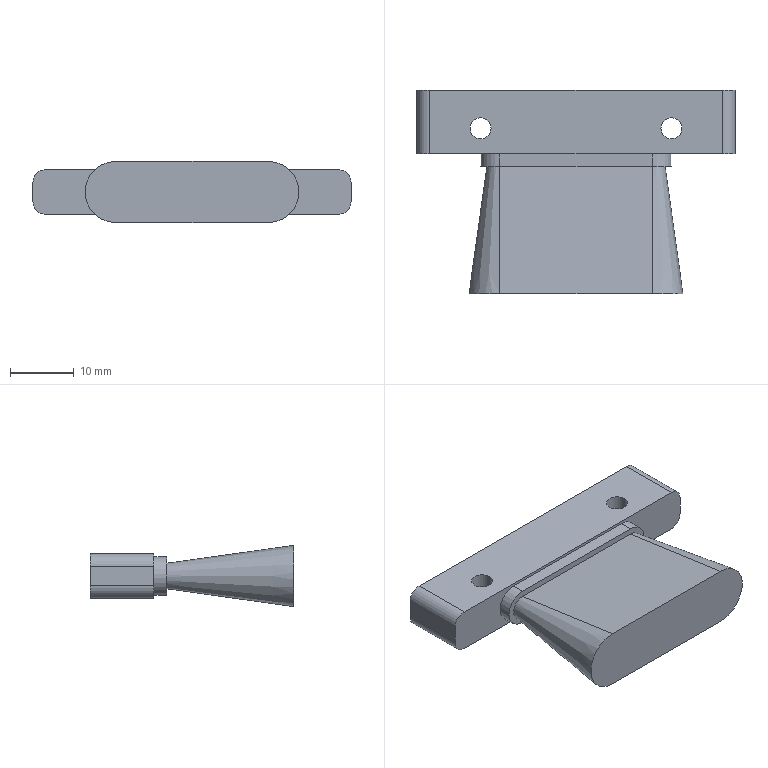Part | SolidWorks | features ICE 2, 3DProfileFeature 1, Extrusion 1, Fillet 1, HoleWzd 1 | 1 solid | 24 faces | box 50 x 32 x 9.622 mm | volume 7730 mm3 | plane 12 | cylinder 10 | cone 2 | commonest cylinder face diameters 3.3 x4 4 x4 6 x2
STEP:
#1=CARTESIAN_POINT('',(16.65,4.,3.5));
#2=VERTEX_POINT('',#1);
#3=CARTESIAN_POINT('',(13.35,4.,3.5));
#4=VERTEX_POINT('',#3);
#5=CARTESIAN_POINT('',(15.,4.,3.5));
#6=DIRECTION('',(0.,0.,-1.));
#7=DIRECTION('',(-1.,0.,0.));
#8=AXIS2_PLACEMENT_3D('',#5,#6,#7);
#9=CIRCLE('',#8,1.65);
#10=EDGE_CURVE('',#2,#4,#9,.T.);
#11=ORIENTED_EDGE('',*,*,#10,.F.);
#12=CARTESIAN_POINT('',(16.65,4.,-3.5));
#13=VERTEX_POINT('',#12);
#14=CARTESIAN_POINT('',(16.65,4.,-3.5));
#15=DIRECTION('',(0.,0.,-1.));
#16=VECTOR('',#15,1000.);
#17=LINE('',#14,#16);
#18=EDGE_CURVE('',#2,#13,#17,.T.);
#19=ORIENTED_EDGE('',*,*,#18,.T.);
#20=CARTESIAN_POINT('',(13.35,4.,-3.5));
#21=VERTEX_POINT('',#20);
#22=CARTESIAN_POINT('',(15.,4.,-3.5));
#23=DIRECTION('',(0.,0.,-1.));
#24=DIRECTION('',(-1.,0.,0.));
#25=AXIS2_PLACEMENT_3D('',#22,#23,#24);
#26=CIRCLE('',#25,1.65);
#27=EDGE_CURVE('',#13,#21,#26,.T.);
#28=ORIENTED_EDGE('',*,*,#27,.T.);
#29=CARTESIAN_POINT('',(13.35,4.,-3.5));
#30=DIRECTION('',(0.,0.,-1.));
#31=VECTOR('',#30,1000.);
#32=LINE('',#29,#31);
#33=EDGE_CURVE('',#4,#21,#32,.T.);
#34=ORIENTED_EDGE('',*,*,#33,.F.);
#35=EDGE_LOOP('',(#11,#19,#28,#34));
#36=FACE_OUTER_BOUND('',#35,.T.);
#37=CARTESIAN_POINT('',(15.,4.,-3.5));
#38=DIRECTION('',(0.,0.,-1.));
#39=DIRECTION('',(-1.,0.,0.));
#40=AXIS2_PLACEMENT_3D('',#37,#38,#39);
#41=CYLINDRICAL_SURFACE('',#40,1.65);
#42=ADVANCED_FACE('',(#36),#41,.F.);
#43=CARTESIAN_POINT('',(-13.35,4.,3.5));
#44=VERTEX_POINT('',#43);
#45=CARTESIAN_POINT('',(-16.65,4.,3.5));
#46=VERTEX_POINT('',#45);
#47=CARTESIAN_POINT('',(-15.,4.,3.5));
#48=DIRECTION('',(0.,0.,-1.));
#49=DIRECTION('',(-1.,0.,0.));
#50=AXIS2_PLACEMENT_3D('',#47,#48,#49);
#51=CIRCLE('',#50,1.65);
#52=EDGE_CURVE('',#44,#46,#51,.T.);
#53=ORIENTED_EDGE('',*,*,#52,.F.);
#54=CARTESIAN_POINT('',(-13.35,4.,-3.5));
#55=VERTEX_POINT('',#54);
#56=CARTESIAN_POINT('',(-13.35,4.,-3.5));
#57=DIRECTION('',(0.,0.,-1.));
#58=VECTOR('',#57,1000.);
#59=LINE('',#56,#58);
#60=EDGE_CURVE('',#44,#55,#59,.T.);
#61=ORIENTED_EDGE('',*,*,#60,.T.);
#62=CARTESIAN_POINT('',(-16.65,4.,-3.5));
#63=VERTEX_POINT('',#62);
#64=CARTESIAN_POINT('',(-15.,4.,-3.5));
#65=DIRECTION('',(0.,0.,-1.));
#66=DIRECTION('',(-1.,0.,0.));
#67=AXIS2_PLACEMENT_3D('',#64,#65,#66);
#68=CIRCLE('',#67,1.65);
#69=EDGE_CURVE('',#55,#63,#68,.T.);
#70=ORIENTED_EDGE('',*,*,#69,.T.);
#71=CARTESIAN_POINT('',(-16.65,4.,-3.5));
#72=DIRECTION('',(0.,0.,-1.));
#73=VECTOR('',#72,1000.);
#74=LINE('',#71,#73);
#75=EDGE_CURVE('',#46,#63,#74,.T.);
#76=ORIENTED_EDGE('',*,*,#75,.F.);
#77=EDGE_LOOP('',(#53,#61,#70,#76));
#78=FACE_OUTER_BOUND('',#77,.T.);
#79=CARTESIAN_POINT('',(-15.,4.,-3.5));
#80=DIRECTION('',(0.,0.,-1.));
#81=DIRECTION('',(-1.,0.,0.));
#82=AXIS2_PLACEMENT_3D('',#79,#80,#81);
#83=CYLINDRICAL_SURFACE('',#82,1.65);
#84=ADVANCED_FACE('',(#78),#83,.F.);
#85=CARTESIAN_POINT('',(-12.,-2.,3.));
#86=VERTEX_POINT('',#85);
#87=CARTESIAN_POINT('',(12.,-2.,3.));
#88=VERTEX_POINT('',#87);
#89=CARTESIAN_POINT('',(0.,-2.,3.));
#90=DIRECTION('',(1.,0.,0.));
#91=VECTOR('',#90,1000.);
#92=LINE('',#89,#91);
#93=EDGE_CURVE('',#86,#88,#92,.T.);
#94=ORIENTED_EDGE('',*,*,#93,.F.);
#95=CARTESIAN_POINT('',(-12.,-2.,-3.));
#96=VERTEX_POINT('',#95);
#97=CARTESIAN_POINT('',(-12.,-2.,0.));
#98=DIRECTION('',(0.,1.,0.));
#99=DIRECTION('',(0.,0.,1.));
#100=AXIS2_PLACEMENT_3D('',#97,#98,#99);
#101=CIRCLE('',#100,3.);
#102=EDGE_CURVE('',#96,#86,#101,.T.);
#103=ORIENTED_EDGE('',*,*,#102,.F.);
#104=CARTESIAN_POINT('',(12.,-2.,-3.));
#105=VERTEX_POINT('',#104);
#106=CARTESIAN_POINT('',(0.,-2.,-3.));
#107=DIRECTION('',(1.,0.,0.));
#108=VECTOR('',#107,1000.);
#109=LINE('',#106,#108);
#110=EDGE_CURVE('',#96,#105,#109,.T.);
#111=ORIENTED_EDGE('',*,*,#110,.T.);
#112=CARTESIAN_POINT('',(12.,-2.,0.));
#113=DIRECTION('',(0.,1.,0.));
#114=DIRECTION('',(0.,0.,1.));
#115=AXIS2_PLACEMENT_3D('',#112,#113,#114);
#116=CIRCLE('',#115,3.);
#117=EDGE_CURVE('',#88,#105,#116,.T.);
#118=ORIENTED_EDGE('',*,*,#117,.F.);
#119=EDGE_LOOP('',(#94,#103,#111,#118));
#120=FACE_OUTER_BOUND('',#119,.T.);
#121=CARTESIAN_POINT('',(12.,-2.,-2.));
#122=VERTEX_POINT('',#121);
#123=CARTESIAN_POINT('',(12.,-2.,2.));
#124=VERTEX_POINT('',#123);
#125=CARTESIAN_POINT('',(12.,-2.,0.));
#126=DIRECTION('',(0.,-1.,0.));
#127=DIRECTION('',(0.,0.,-1.));
#128=AXIS2_PLACEMENT_3D('',#125,#126,#127);
#129=CIRCLE('',#128,2.);
#130=EDGE_CURVE('',#122,#124,#129,.T.);
#131=ORIENTED_EDGE('',*,*,#130,.F.);
#132=CARTESIAN_POINT('',(-12.,-2.,-2.));
#133=VERTEX_POINT('',#132);
#134=CARTESIAN_POINT('',(-12.,-2.,-2.));
#135=DIRECTION('',(1.,0.,0.));
#136=VECTOR('',#135,1000.);
#137=LINE('',#134,#136);
#138=EDGE_CURVE('',#133,#122,#137,.T.);
#139=ORIENTED_EDGE('',*,*,#138,.F.);
#140=CARTESIAN_POINT('',(-12.,-2.,2.));
#141=VERTEX_POINT('',#140);
#142=CARTESIAN_POINT('',(-12.,-2.,0.));
#143=DIRECTION('',(0.,-1.,0.));
#144=DIRECTION('',(0.,0.,-1.));
#145=AXIS2_PLACEMENT_3D('',#142,#143,#144);
#146=CIRCLE('',#145,2.);
#147=EDGE_CURVE('',#141,#133,#146,.T.);
#148=ORIENTED_EDGE('',*,*,#147,.F.);
#149=CARTESIAN_POINT('',(12.,-2.,2.));
#150=DIRECTION('',(-1.,0.,0.));
#151=VECTOR('',#150,1000.);
#152=LINE('',#149,#151);
#153=EDGE_CURVE('',#124,#141,#152,.T.);
#154=ORIENTED_EDGE('',*,*,#153,.F.);
#155=EDGE_LOOP('',(#131,#139,#148,#154));
#156=FACE_BOUND('',#155,.T.);
#157=CARTESIAN_POINT('',(0.,-2.,0.));
#158=DIRECTION('',(0.,1.,0.));
#159=DIRECTION('',(0.,0.,1.));
#160=AXIS2_PLACEMENT_3D('',#157,#158,#159);
#161=PLANE('',#160);
#162=ADVANCED_FACE('',(#120,#156),#161,.F.);
#163=CARTESIAN_POINT('',(15.,4.,3.5));
#164=DIRECTION('',(0.,0.,-1.));
#165=DIRECTION('',(-1.,0.,0.));
#166=AXIS2_PLACEMENT_3D('',#163,#164,#165);
#167=CIRCLE('',#166,1.65);
#168=EDGE_CURVE('',#4,#2,#167,.T.);
#169=ORIENTED_EDGE('',*,*,#168,.T.);
#170=ORIENTED_EDGE('',*,*,#10,.T.);
#171=EDGE_LOOP('',(#169,#170));
#172=FACE_BOUND('',#171,.T.);
#173=CARTESIAN_POINT('',(-15.,4.,3.5));
#174=DIRECTION('',(0.,0.,-1.));
#175=DIRECTION('',(-1.,0.,0.));
#176=AXIS2_PLACEMENT_3D('',#173,#174,#175);
#177=CIRCLE('',#176,1.65);
#178=EDGE_CURVE('',#46,#44,#177,.T.);
#179=ORIENTED_EDGE('',*,*,#178,.T.);
#180=ORIENTED_EDGE('',*,*,#52,.T.);
#181=EDGE_LOOP('',(#179,#180));
#182=FACE_BOUND('',#181,.T.);
#183=CARTESIAN_POINT('',(-23.,0.,3.5));
#184=VERTEX_POINT('',#183);
#185=CARTESIAN_POINT('',(23.,0.,3.5));
#186=VERTEX_POINT('',#185);
#187=CARTESIAN_POINT('',(0.,0.,3.5));
#188=DIRECTION('',(1.,0.,0.));
#189=VECTOR('',#188,1000.);
#190=LINE('',#187,#189);
#191=EDGE_CURVE('',#184,#186,#190,.T.);
#192=ORIENTED_EDGE('',*,*,#191,.T.);
#193=CARTESIAN_POINT('',(23.,10.,3.5));
#194=VERTEX_POINT('',#193);
#195=CARTESIAN_POINT('',(23.,10.,3.5));
#196=DIRECTION('',(0.,1.,0.));
#197=VECTOR('',#196,1000.);
#198=LINE('',#195,#197);
#199=EDGE_CURVE('',#186,#194,#198,.T.);
#200=ORIENTED_EDGE('',*,*,#199,.T.);
#201=CARTESIAN_POINT('',(-23.,10.,3.5));
#202=VERTEX_POINT('',#201);
#203=CARTESIAN_POINT('',(0.,10.,3.5));
#204=DIRECTION('',(1.,0.,0.));
#205=VECTOR('',#204,1000.);
#206=LINE('',#203,#205);
#207=EDGE_CURVE('',#202,#194,#206,.T.);
#208=ORIENTED_EDGE('',*,*,#207,.F.);
#209=CARTESIAN_POINT('',(-23.,10.,3.5));
#210=DIRECTION('',(0.,-1.,0.));
#211=VECTOR('',#210,1000.);
#212=LINE('',#209,#211);
#213=EDGE_CURVE('',#202,#184,#212,.T.);
#214=ORIENTED_EDGE('',*,*,#213,.T.);
#215=EDGE_LOOP('',(#192,#200,#208,#214));
#216=FACE_OUTER_BOUND('',#215,.T.);
#217=CARTESIAN_POINT('',(0.,10.,3.5));
#218=DIRECTION('',(0.,0.,-1.));
#219=DIRECTION('',(-1.,0.,0.));
#220=AXIS2_PLACEMENT_3D('',#217,#218,#219);
#221=PLANE('',#220);
#222=ADVANCED_FACE('',(#172,#182,#216),#221,.F.);
#223=CARTESIAN_POINT('',(25.,0.,1.5));
#224=VERTEX_POINT('',#223);
#225=CARTESIAN_POINT('',(25.,0.,-1.5));
#226=VERTEX_POINT('',#225);
#227=CARTESIAN_POINT('',(25.,0.,0.));
#228=DIRECTION('',(0.,0.,-1.));
#229=VECTOR('',#228,1000.);
#230=LINE('',#227,#229);
#231=EDGE_CURVE('',#224,#226,#230,.T.);
#232=ORIENTED_EDGE('',*,*,#231,.T.);
#233=CARTESIAN_POINT('',(25.,10.,-1.5));
#234=VERTEX_POINT('',#233);
#235=CARTESIAN_POINT('',(25.,10.,-1.5));
#236=DIRECTION('',(0.,1.,0.));
#237=VECTOR('',#236,1000.);
#238=LINE('',#235,#237);
#239=EDGE_CURVE('',#226,#234,#238,.T.);
#240=ORIENTED_EDGE('',*,*,#239,.T.);
#241=CARTESIAN_POINT('',(25.,10.,1.5));
#242=VERTEX_POINT('',#241);
#243=CARTESIAN_POINT('',(25.,10.,0.));
#244=DIRECTION('',(0.,0.,-1.));
#245=VECTOR('',#244,1000.);
#246=LINE('',#243,#245);
#247=EDGE_CURVE('',#242,#234,#246,.T.);
#248=ORIENTED_EDGE('',*,*,#247,.F.);
#249=CARTESIAN_POINT('',(25.,10.,1.5));
#250=DIRECTION('',(0.,-1.,0.));
#251=VECTOR('',#250,1000.);
#252=LINE('',#249,#251);
#253=EDGE_CURVE('',#242,#224,#252,.T.);
#254=ORIENTED_EDGE('',*,*,#253,.T.);
#255=EDGE_LOOP('',(#232,#240,#248,#254));
#256=FACE_OUTER_BOUND('',#255,.T.);
#257=CARTESIAN_POINT('',(25.,10.,0.));
#258=DIRECTION('',(-1.,0.,0.));
#259=DIRECTION('',(0.,0.,1.));
#260=AXIS2_PLACEMENT_3D('',#257,#258,#259);
#261=PLANE('',#260);
#262=ADVANCED_FACE('',(#256),#261,.F.);
#263=CARTESIAN_POINT('',(15.,4.,-3.5));
#264=DIRECTION('',(0.,0.,-1.));
#265=DIRECTION('',(-1.,0.,0.));
#266=AXIS2_PLACEMENT_3D('',#263,#264,#265);
#267=CIRCLE('',#266,1.65);
#268=EDGE_CURVE('',#21,#13,#267,.T.);
#269=ORIENTED_EDGE('',*,*,#268,.F.);
#270=ORIENTED_EDGE('',*,*,#27,.F.);
#271=EDGE_LOOP('',(#269,#270));
#272=FACE_BOUND('',#271,.T.);
#273=CARTESIAN_POINT('',(-15.,4.,-3.5));
#274=DIRECTION('',(0.,0.,-1.));
#275=DIRECTION('',(-1.,0.,0.));
#276=AXIS2_PLACEMENT_3D('',#273,#274,#275);
#277=CIRCLE('',#276,1.65);
#278=EDGE_CURVE('',#63,#55,#277,.T.);
#279=ORIENTED_EDGE('',*,*,#278,.F.);
#280=ORIENTED_EDGE('',*,*,#69,.F.);
#281=EDGE_LOOP('',(#279,#280));
#282=FACE_BOUND('',#281,.T.);
#283=CARTESIAN_POINT('',(23.,0.,-3.5));
#284=VERTEX_POINT('',#283);
#285=CARTESIAN_POINT('',(-23.,0.,-3.5));
#286=VERTEX_POINT('',#285);
#287=CARTESIAN_POINT('',(0.,0.,-3.5));
#288=DIRECTION('',(-1.,0.,0.));
#289=VECTOR('',#288,1000.);
#290=LINE('',#287,#289);
#291=EDGE_CURVE('',#284,#286,#290,.T.);
#292=ORIENTED_EDGE('',*,*,#291,.T.);
#293=CARTESIAN_POINT('',(-23.,10.,-3.5));
#294=VERTEX_POINT('',#293);
#295=CARTESIAN_POINT('',(-23.,10.,-3.5));
#296=DIRECTION('',(0.,1.,0.));
#297=VECTOR('',#296,1000.);
#298=LINE('',#295,#297);
#299=EDGE_CURVE('',#286,#294,#298,.T.);
#300=ORIENTED_EDGE('',*,*,#299,.T.);
#301=CARTESIAN_POINT('',(23.,10.,-3.5));
#302=VERTEX_POINT('',#301);
#303=CARTESIAN_POINT('',(0.,10.,-3.5));
#304=DIRECTION('',(-1.,0.,0.));
#305=VECTOR('',#304,1000.);
#306=LINE('',#303,#305);
#307=EDGE_CURVE('',#302,#294,#306,.T.);
#308=ORIENTED_EDGE('',*,*,#307,.F.);
#309=CARTESIAN_POINT('',(23.,10.,-3.5));
#310=DIRECTION('',(0.,-1.,0.));
#311=VECTOR('',#310,1000.);
#312=LINE('',#309,#311);
#313=EDGE_CURVE('',#302,#284,#312,.T.);
#314=ORIENTED_EDGE('',*,*,#313,.T.);
#315=EDGE_LOOP('',(#292,#300,#308,#314));
#316=FACE_OUTER_BOUND('',#315,.T.);
#317=CARTESIAN_POINT('',(0.,10.,-3.5));
#318=DIRECTION('',(0.,0.,1.));
#319=DIRECTION('',(1.,0.,0.));
#320=AXIS2_PLACEMENT_3D('',#317,#318,#319);
#321=PLANE('',#320);
#322=ADVANCED_FACE('',(#272,#282,#316),#321,.F.);
#323=CARTESIAN_POINT('',(-25.,10.,-1.5));
#324=VERTEX_POINT('',#323);
#325=CARTESIAN_POINT('',(-25.,10.,1.5));
#326=VERTEX_POINT('',#325);
#327=CARTESIAN_POINT('',(-25.,10.,0.));
#328=DIRECTION('',(0.,0.,1.));
#329=VECTOR('',#328,1000.);
#330=LINE('',#327,#329);
#331=EDGE_CURVE('',#324,#326,#330,.T.);
#332=ORIENTED_EDGE('',*,*,#331,.F.);
#333=CARTESIAN_POINT('',(-25.,0.,-1.5));
#334=VERTEX_POINT('',#333);
#335=CARTESIAN_POINT('',(-25.,10.,-1.5));
#336=DIRECTION('',(0.,-1.,0.));
#337=VECTOR('',#336,1000.);
#338=LINE('',#335,#337);
#339=EDGE_CURVE('',#324,#334,#338,.T.);
#340=ORIENTED_EDGE('',*,*,#339,.T.);
#341=CARTESIAN_POINT('',(-25.,0.,1.5));
#342=VERTEX_POINT('',#341);
#343=CARTESIAN_POINT('',(-25.,0.,0.));
#344=DIRECTION('',(0.,0.,1.));
#345=VECTOR('',#344,1000.);
#346=LINE('',#343,#345);
#347=EDGE_CURVE('',#334,#342,#346,.T.);
#348=ORIENTED_EDGE('',*,*,#347,.T.);
#349=CARTESIAN_POINT('',(-25.,10.,1.5));
#350=DIRECTION('',(0.,1.,0.));
#351=VECTOR('',#350,1000.);
#352=LINE('',#349,#351);
#353=EDGE_CURVE('',#342,#326,#352,.T.);
#354=ORIENTED_EDGE('',*,*,#353,.T.);
#355=EDGE_LOOP('',(#332,#340,#348,#354));
#356=FACE_OUTER_BOUND('',#355,.T.);
#357=CARTESIAN_POINT('',(-25.,10.,0.));
#358=DIRECTION('',(1.,0.,0.));
#359=DIRECTION('',(0.,0.,-1.));
#360=AXIS2_PLACEMENT_3D('',#357,#358,#359);
#361=PLANE('',#360);
#362=ADVANCED_FACE('',(#356),#361,.F.);
#363=ORIENTED_EDGE('',*,*,#307,.T.);
#364=CARTESIAN_POINT('',(-23.,10.,-1.5));
#365=DIRECTION('',(0.,1.,0.));
#366=DIRECTION('',(0.,0.,1.));
#367=AXIS2_PLACEMENT_3D('',#364,#365,#366);
#368=CIRCLE('',#367,2.);
#369=EDGE_CURVE('',#294,#324,#368,.T.);
#370=ORIENTED_EDGE('',*,*,#369,.T.);
#371=ORIENTED_EDGE('',*,*,#331,.T.);
#372=CARTESIAN_POINT('',(-23.,10.,1.5));
#373=DIRECTION('',(0.,1.,0.));
#374=DIRECTION('',(0.,0.,1.));
#375=AXIS2_PLACEMENT_3D('',#372,#373,#374);
#376=CIRCLE('',#375,2.);
#377=EDGE_CURVE('',#326,#202,#376,.T.);
#378=ORIENTED_EDGE('',*,*,#377,.T.);
#379=ORIENTED_EDGE('',*,*,#207,.T.);
#380=CARTESIAN_POINT('',(23.,10.,1.5));
#381=DIRECTION('',(0.,1.,0.));
#382=DIRECTION('',(0.,0.,1.));
#383=AXIS2_PLACEMENT_3D('',#380,#381,#382);
#384=CIRCLE('',#383,2.);
#385=EDGE_CURVE('',#194,#242,#384,.T.);
#386=ORIENTED_EDGE('',*,*,#385,.T.);
#387=ORIENTED_EDGE('',*,*,#247,.T.);
#388=CARTESIAN_POINT('',(23.,10.,-1.5));
#389=DIRECTION('',(0.,1.,0.));
#390=DIRECTION('',(0.,0.,1.));
#391=AXIS2_PLACEMENT_3D('',#388,#389,#390);
#392=CIRCLE('',#391,2.);
#393=EDGE_CURVE('',#234,#302,#392,.T.);
#394=ORIENTED_EDGE('',*,*,#393,.T.);
#395=EDGE_LOOP('',(#363,#370,#371,#378,#379,#386,#387,#394));
#396=FACE_OUTER_BOUND('',#395,.T.);
#397=CARTESIAN_POINT('',(0.,10.,0.));
#398=DIRECTION('',(0.,1.,0.));
#399=DIRECTION('',(0.,0.,1.));
#400=AXIS2_PLACEMENT_3D('',#397,#398,#399);
#401=PLANE('',#400);
#402=ADVANCED_FACE('',(#396),#401,.T.);
#403=CARTESIAN_POINT('',(-12.,0.,-3.));
#404=VERTEX_POINT('',#403);
#405=CARTESIAN_POINT('',(-12.,0.,3.));
#406=VERTEX_POINT('',#405);
#407=CARTESIAN_POINT('',(-12.,0.,0.));
#408=DIRECTION('',(0.,1.,0.));
#409=DIRECTION('',(0.,0.,1.));
#410=AXIS2_PLACEMENT_3D('',#407,#408,#409);
#411=CIRCLE('',#410,3.);
#412=EDGE_CURVE('',#404,#406,#411,.T.);
#413=ORIENTED_EDGE('',*,*,#412,.T.);
#414=CARTESIAN_POINT('',(12.,0.,3.));
#415=VERTEX_POINT('',#414);
#416=CARTESIAN_POINT('',(0.,0.,3.));
#417=DIRECTION('',(1.,0.,0.));
#418=VECTOR('',#417,1000.);
#419=LINE('',#416,#418);
#420=EDGE_CURVE('',#406,#415,#419,.T.);
#421=ORIENTED_EDGE('',*,*,#420,.T.);
#422=CARTESIAN_POINT('',(12.,0.,-3.));
#423=VERTEX_POINT('',#422);
#424=CARTESIAN_POINT('',(12.,0.,0.));
#425=DIRECTION('',(0.,1.,0.));
#426=DIRECTION('',(0.,0.,1.));
#427=AXIS2_PLACEMENT_3D('',#424,#425,#426);
#428=CIRCLE('',#427,3.);
#429=EDGE_CURVE('',#415,#423,#428,.T.);
#430=ORIENTED_EDGE('',*,*,#429,.T.);
#431=CARTESIAN_POINT('',(0.,0.,-3.));
#432=DIRECTION('',(1.,0.,0.));
#433=VECTOR('',#432,1000.);
#434=LINE('',#431,#433);
#435=EDGE_CURVE('',#404,#423,#434,.T.);
#436=ORIENTED_EDGE('',*,*,#435,.F.);
#437=EDGE_LOOP('',(#413,#421,#430,#436));
#438=FACE_BOUND('',#437,.T.);
#439=ORIENTED_EDGE('',*,*,#347,.F.);
#440=CARTESIAN_POINT('',(-23.,0.,-1.5));
#441=DIRECTION('',(0.,-1.,0.));
#442=DIRECTION('',(0.,0.,1.));
#443=AXIS2_PLACEMENT_3D('',#440,#441,#442);
#444=CIRCLE('',#443,2.);
#445=EDGE_CURVE('',#334,#286,#444,.T.);
#446=ORIENTED_EDGE('',*,*,#445,.T.);
#447=ORIENTED_EDGE('',*,*,#291,.F.);
#448=CARTESIAN_POINT('',(23.,0.,-1.5));
#449=DIRECTION('',(0.,-1.,0.));
#450=DIRECTION('',(0.,0.,1.));
#451=AXIS2_PLACEMENT_3D('',#448,#449,#450);
#452=CIRCLE('',#451,2.);
#453=EDGE_CURVE('',#284,#226,#452,.T.);
#454=ORIENTED_EDGE('',*,*,#453,.T.);
#455=ORIENTED_EDGE('',*,*,#231,.F.);
#456=CARTESIAN_POINT('',(23.,0.,1.5));
#457=DIRECTION('',(0.,-1.,0.));
#458=DIRECTION('',(0.,0.,1.));
#459=AXIS2_PLACEMENT_3D('',#456,#457,#458);
#460=CIRCLE('',#459,2.);
#461=EDGE_CURVE('',#224,#186,#460,.T.);
#462=ORIENTED_EDGE('',*,*,#461,.T.);
#463=ORIENTED_EDGE('',*,*,#191,.F.);
#464=CARTESIAN_POINT('',(-23.,0.,1.5));
#465=DIRECTION('',(0.,-1.,0.));
#466=DIRECTION('',(0.,0.,1.));
#467=AXIS2_PLACEMENT_3D('',#464,#465,#466);
#468=CIRCLE('',#467,2.);
#469=EDGE_CURVE('',#184,#342,#468,.T.);
#470=ORIENTED_EDGE('',*,*,#469,.T.);
#471=EDGE_LOOP('',(#439,#446,#447,#454,#455,#462,#463,#470));
#472=FACE_OUTER_BOUND('',#471,.T.);
#473=CARTESIAN_POINT('',(0.,0.,0.));
#474=DIRECTION('',(0.,1.,0.));
#475=DIRECTION('',(0.,0.,1.));
#476=AXIS2_PLACEMENT_3D('',#473,#474,#475);
#477=PLANE('',#476);
#478=ADVANCED_FACE('',(#438,#472),#477,.F.);
#479=ORIENTED_EDGE('',*,*,#420,.F.);
#480=CARTESIAN_POINT('',(-12.,-2.,3.));
#481=DIRECTION('',(0.,1.,0.));
#482=VECTOR('',#481,1000.);
#483=LINE('',#480,#482);
#484=EDGE_CURVE('',#86,#406,#483,.T.);
#485=ORIENTED_EDGE('',*,*,#484,.F.);
#486=ORIENTED_EDGE('',*,*,#93,.T.);
#487=CARTESIAN_POINT('',(12.,-2.,3.));
#488=DIRECTION('',(0.,1.,0.));
#489=VECTOR('',#488,1000.);
#490=LINE('',#487,#489);
#491=EDGE_CURVE('',#88,#415,#490,.T.);
#492=ORIENTED_EDGE('',*,*,#491,.T.);
#493=EDGE_LOOP('',(#479,#485,#486,#492));
#494=FACE_OUTER_BOUND('',#493,.T.);
#495=CARTESIAN_POINT('',(0.,-2.,3.));
#496=DIRECTION('',(0.,0.,1.));
#497=DIRECTION('',(1.,0.,0.));
#498=AXIS2_PLACEMENT_3D('',#495,#496,#497);
#499=PLANE('',#498);
#500=ADVANCED_FACE('',(#494),#499,.T.);
#501=ORIENTED_EDGE('',*,*,#412,.F.);
#502=CARTESIAN_POINT('',(-12.,-2.,-3.));
#503=DIRECTION('',(0.,1.,0.));
#504=VECTOR('',#503,1000.);
#505=LINE('',#502,#504);
#506=EDGE_CURVE('',#96,#404,#505,.T.);
#507=ORIENTED_EDGE('',*,*,#506,.F.);
#508=ORIENTED_EDGE('',*,*,#102,.T.);
#509=ORIENTED_EDGE('',*,*,#484,.T.);
#510=EDGE_LOOP('',(#501,#507,#508,#509));
#511=FACE_OUTER_BOUND('',#510,.T.);
#512=CARTESIAN_POINT('',(-12.,-2.,0.));
#513=DIRECTION('',(0.,1.,0.));
#514=DIRECTION('',(0.,0.,1.));
#515=AXIS2_PLACEMENT_3D('',#512,#513,#514);
#516=CYLINDRICAL_SURFACE('',#515,3.);
#517=ADVANCED_FACE('',(#511),#516,.T.);
#518=ORIENTED_EDGE('',*,*,#435,.T.);
#519=CARTESIAN_POINT('',(12.,-2.,-3.));
#520=DIRECTION('',(0.,1.,0.));
#521=VECTOR('',#520,1000.);
#522=LINE('',#519,#521);
#523=EDGE_CURVE('',#105,#423,#522,.T.);
#524=ORIENTED_EDGE('',*,*,#523,.F.);
#525=ORIENTED_EDGE('',*,*,#110,.F.);
#526=ORIENTED_EDGE('',*,*,#506,.T.);
#527=EDGE_LOOP('',(#518,#524,#525,#526));
#528=FACE_OUTER_BOUND('',#527,.T.);
#529=CARTESIAN_POINT('',(0.,-2.,-3.));
#530=DIRECTION('',(0.,0.,1.));
#531=DIRECTION('',(1.,0.,0.));
#532=AXIS2_PLACEMENT_3D('',#529,#530,#531);
#533=PLANE('',#532);
#534=ADVANCED_FACE('',(#528),#533,.F.);
#535=ORIENTED_EDGE('',*,*,#429,.F.);
#536=ORIENTED_EDGE('',*,*,#491,.F.);
#537=ORIENTED_EDGE('',*,*,#117,.T.);
#538=ORIENTED_EDGE('',*,*,#523,.T.);
#539=EDGE_LOOP('',(#535,#536,#537,#538));
#540=FACE_OUTER_BOUND('',#539,.T.);
#541=CARTESIAN_POINT('',(12.,-2.,0.));
#542=DIRECTION('',(0.,1.,0.));
#543=DIRECTION('',(0.,0.,1.));
#544=AXIS2_PLACEMENT_3D('',#541,#542,#543);
#545=CYLINDRICAL_SURFACE('',#544,3.);
#546=ADVANCED_FACE('',(#540),#545,.T.);
#547=ORIENTED_EDGE('',*,*,#130,.T.);
#548=CARTESIAN_POINT('',(12.,-22.,4.811));
#549=VERTEX_POINT('',#548);
#550=CARTESIAN_POINT('',(12.,-2.,2.));
#551=DIRECTION('',(0.,0.9903,-0.1392));
#552=VECTOR('',#551,1000.);
#553=LINE('',#550,#552);
#554=EDGE_CURVE('',#549,#124,#553,.T.);
#555=ORIENTED_EDGE('',*,*,#554,.F.);
#556=CARTESIAN_POINT('',(12.,-22.,-4.811));
#557=VERTEX_POINT('',#556);
#558=CARTESIAN_POINT('',(12.,-22.,0.));
#559=DIRECTION('',(0.,-1.,0.));
#560=DIRECTION('',(0.,0.,-1.));
#561=AXIS2_PLACEMENT_3D('',#558,#559,#560);
#562=CIRCLE('',#561,4.811);
#563=EDGE_CURVE('',#557,#549,#562,.T.);
#564=ORIENTED_EDGE('',*,*,#563,.F.);
#565=CARTESIAN_POINT('',(12.,-2.,-2.));
#566=DIRECTION('',(0.,0.9903,0.1392));
#567=VECTOR('',#566,1000.);
#568=LINE('',#565,#567);
#569=EDGE_CURVE('',#557,#122,#568,.T.);
#570=ORIENTED_EDGE('',*,*,#569,.T.);
#571=EDGE_LOOP('',(#547,#555,#564,#570));
#572=FACE_OUTER_BOUND('',#571,.T.);
#573=CARTESIAN_POINT('',(12.,-2.,0.));
#574=DIRECTION('',(0.,-1.,0.));
#575=DIRECTION('',(0.,0.,-1.));
#576=AXIS2_PLACEMENT_3D('',#573,#574,#575);
#577=CONICAL_SURFACE('',#576,2.,0.1396);
#578=ADVANCED_FACE('',(#572),#577,.T.);
#579=ORIENTED_EDGE('',*,*,#153,.T.);
#580=CARTESIAN_POINT('',(-12.,-22.,4.811));
#581=VERTEX_POINT('',#580);
#582=CARTESIAN_POINT('',(-12.,-2.,2.));
#583=DIRECTION('',(0.,0.9903,-0.1392));
#584=VECTOR('',#583,1000.);
#585=LINE('',#582,#584);
#586=EDGE_CURVE('',#581,#141,#585,.T.);
#587=ORIENTED_EDGE('',*,*,#586,.F.);
#588=CARTESIAN_POINT('',(12.,-22.,4.811));
#589=DIRECTION('',(-1.,0.,0.));
#590=VECTOR('',#589,1000.);
#591=LINE('',#588,#590);
#592=EDGE_CURVE('',#549,#581,#591,.T.);
#593=ORIENTED_EDGE('',*,*,#592,.F.);
#594=ORIENTED_EDGE('',*,*,#554,.T.);
#595=EDGE_LOOP('',(#579,#587,#593,#594));
#596=FACE_OUTER_BOUND('',#595,.T.);
#597=CARTESIAN_POINT('',(12.,-2.,2.));
#598=DIRECTION('',(0.,0.1392,0.9903));
#599=DIRECTION('',(0.,-0.9903,0.1392));
#600=AXIS2_PLACEMENT_3D('',#597,#598,#599);
#601=PLANE('',#600);
#602=ADVANCED_FACE('',(#596),#601,.T.);
#603=ORIENTED_EDGE('',*,*,#147,.T.);
#604=CARTESIAN_POINT('',(-12.,-22.,-4.811));
#605=VERTEX_POINT('',#604);
#606=CARTESIAN_POINT('',(-12.,-2.,-2.));
#607=DIRECTION('',(0.,0.9903,0.1392));
#608=VECTOR('',#607,1000.);
#609=LINE('',#606,#608);
#610=EDGE_CURVE('',#605,#133,#609,.T.);
#611=ORIENTED_EDGE('',*,*,#610,.F.);
#612=CARTESIAN_POINT('',(-12.,-22.,0.));
#613=DIRECTION('',(0.,-1.,0.));
#614=DIRECTION('',(0.,0.,-1.));
#615=AXIS2_PLACEMENT_3D('',#612,#613,#614);
#616=CIRCLE('',#615,4.811);
#617=EDGE_CURVE('',#581,#605,#616,.T.);
#618=ORIENTED_EDGE('',*,*,#617,.F.);
#619=ORIENTED_EDGE('',*,*,#586,.T.);
#620=EDGE_LOOP('',(#603,#611,#618,#619));
#621=FACE_OUTER_BOUND('',#620,.T.);
#622=CARTESIAN_POINT('',(-12.,-2.,0.));
#623=DIRECTION('',(0.,-1.,0.));
#624=DIRECTION('',(0.,0.,-1.));
#625=AXIS2_PLACEMENT_3D('',#622,#623,#624);
#626=CONICAL_SURFACE('',#625,2.,0.1396);
#627=ADVANCED_FACE('',(#621),#626,.T.);
#628=ORIENTED_EDGE('',*,*,#138,.T.);
#629=ORIENTED_EDGE('',*,*,#569,.F.);
#630=CARTESIAN_POINT('',(-12.,-22.,-4.811));
#631=DIRECTION('',(1.,0.,0.));
#632=VECTOR('',#631,1000.);
#633=LINE('',#630,#632);
#634=EDGE_CURVE('',#605,#557,#633,.T.);
#635=ORIENTED_EDGE('',*,*,#634,.F.);
#636=ORIENTED_EDGE('',*,*,#610,.T.);
#637=EDGE_LOOP('',(#628,#629,#635,#636));
#638=FACE_OUTER_BOUND('',#637,.T.);
#639=CARTESIAN_POINT('',(-12.,-2.,-2.));
#640=DIRECTION('',(0.,0.1392,-0.9903));
#641=DIRECTION('',(0.,0.9903,0.1392));
#642=AXIS2_PLACEMENT_3D('',#639,#640,#641);
#643=PLANE('',#642);
#644=ADVANCED_FACE('',(#638),#643,.T.);
#645=ORIENTED_EDGE('',*,*,#563,.T.);
#646=ORIENTED_EDGE('',*,*,#592,.T.);
#647=ORIENTED_EDGE('',*,*,#617,.T.);
#648=ORIENTED_EDGE('',*,*,#634,.T.);
#649=EDGE_LOOP('',(#645,#646,#647,#648));
#650=FACE_OUTER_BOUND('',#649,.T.);
#651=CARTESIAN_POINT('',(12.,-22.,0.));
#652=DIRECTION('',(0.,-1.,0.));
#653=DIRECTION('',(0.,0.,-1.));
#654=AXIS2_PLACEMENT_3D('',#651,#652,#653);
#655=PLANE('',#654);
#656=ADVANCED_FACE('',(#650),#655,.T.);
#657=ORIENTED_EDGE('',*,*,#369,.F.);
#658=ORIENTED_EDGE('',*,*,#299,.F.);
#659=ORIENTED_EDGE('',*,*,#445,.F.);
#660=ORIENTED_EDGE('',*,*,#339,.F.);
#661=EDGE_LOOP('',(#657,#658,#659,#660));
#662=FACE_OUTER_BOUND('',#661,.T.);
#663=CARTESIAN_POINT('',(-23.,10.,-1.5));
#664=DIRECTION('',(0.,-1.,0.));
#665=DIRECTION('',(0.,0.,-1.));
#666=AXIS2_PLACEMENT_3D('',#663,#664,#665);
#667=CYLINDRICAL_SURFACE('',#666,2.);
#668=ADVANCED_FACE('',(#662),#667,.T.);
#669=ORIENTED_EDGE('',*,*,#393,.F.);
#670=ORIENTED_EDGE('',*,*,#239,.F.);
#671=ORIENTED_EDGE('',*,*,#453,.F.);
#672=ORIENTED_EDGE('',*,*,#313,.F.);
#673=EDGE_LOOP('',(#669,#670,#671,#672));
#674=FACE_OUTER_BOUND('',#673,.T.);
#675=CARTESIAN_POINT('',(23.,10.,-1.5));
#676=DIRECTION('',(0.,-1.,0.));
#677=DIRECTION('',(0.,0.,-1.));
#678=AXIS2_PLACEMENT_3D('',#675,#676,#677);
#679=CYLINDRICAL_SURFACE('',#678,2.);
#680=ADVANCED_FACE('',(#674),#679,.T.);
#681=ORIENTED_EDGE('',*,*,#385,.F.);
#682=ORIENTED_EDGE('',*,*,#199,.F.);
#683=ORIENTED_EDGE('',*,*,#461,.F.);
#684=ORIENTED_EDGE('',*,*,#253,.F.);
#685=EDGE_LOOP('',(#681,#682,#683,#684));
#686=FACE_OUTER_BOUND('',#685,.T.);
#687=CARTESIAN_POINT('',(23.,10.,1.5));
#688=DIRECTION('',(0.,-1.,0.));
#689=DIRECTION('',(0.,0.,-1.));
#690=AXIS2_PLACEMENT_3D('',#687,#688,#689);
#691=CYLINDRICAL_SURFACE('',#690,2.);
#692=ADVANCED_FACE('',(#686),#691,.T.);
#693=ORIENTED_EDGE('',*,*,#377,.F.);
#694=ORIENTED_EDGE('',*,*,#353,.F.);
#695=ORIENTED_EDGE('',*,*,#469,.F.);
#696=ORIENTED_EDGE('',*,*,#213,.F.);
#697=EDGE_LOOP('',(#693,#694,#695,#696));
#698=FACE_OUTER_BOUND('',#697,.T.);
#699=CARTESIAN_POINT('',(-23.,10.,1.5));
#700=DIRECTION('',(0.,-1.,0.));
#701=DIRECTION('',(0.,0.,-1.));
#702=AXIS2_PLACEMENT_3D('',#699,#700,#701);
#703=CYLINDRICAL_SURFACE('',#702,2.);
#704=ADVANCED_FACE('',(#698),#703,.T.);
#705=ORIENTED_EDGE('',*,*,#60,.F.);
#706=ORIENTED_EDGE('',*,*,#178,.F.);
#707=ORIENTED_EDGE('',*,*,#75,.T.);
#708=ORIENTED_EDGE('',*,*,#278,.T.);
#709=EDGE_LOOP('',(#705,#706,#707,#708));
#710=FACE_OUTER_BOUND('',#709,.T.);
#711=CARTESIAN_POINT('',(-15.,4.,-3.5));
#712=DIRECTION('',(0.,0.,-1.));
#713=DIRECTION('',(-1.,0.,0.));
#714=AXIS2_PLACEMENT_3D('',#711,#712,#713);
#715=CYLINDRICAL_SURFACE('',#714,1.65);
#716=ADVANCED_FACE('',(#710),#715,.F.);
#717=ORIENTED_EDGE('',*,*,#18,.F.);
#718=ORIENTED_EDGE('',*,*,#168,.F.);
#719=ORIENTED_EDGE('',*,*,#33,.T.);
#720=ORIENTED_EDGE('',*,*,#268,.T.);
#721=EDGE_LOOP('',(#717,#718,#719,#720));
#722=FACE_OUTER_BOUND('',#721,.T.);
#723=CARTESIAN_POINT('',(15.,4.,-3.5));
#724=DIRECTION('',(0.,0.,-1.));
#725=DIRECTION('',(-1.,0.,0.));
#726=AXIS2_PLACEMENT_3D('',#723,#724,#725);
#727=CYLINDRICAL_SURFACE('',#726,1.65);
#728=ADVANCED_FACE('',(#722),#727,.F.);
#729=CLOSED_SHELL('',(#42,#84,#162,#222,#262,#322,#362,#402,#478,#500,#517,#534,#546,#578,#602,#627,#644,#656,#668,#680,#692,#704,#716,#728));
#730=MANIFOLD_SOLID_BREP('',#729);
#731=CARTESIAN_POINT('',(0.,0.,0.));
#732=DIRECTION('',(0.,0.,1.));
#733=DIRECTION('',(1.,0.,0.));
#734=AXIS2_PLACEMENT_3D('',#731,#732,#733);
#735=(LENGTH_UNIT()NAMED_UNIT(*)SI_UNIT(.MILLI.,.METRE.));
#736=UNCERTAINTY_MEASURE_WITH_UNIT(LENGTH_MEASURE(0.00001),#735,'','');
#737=(NAMED_UNIT(*)PLANE_ANGLE_UNIT()SI_UNIT($,.RADIAN.));
#738=(NAMED_UNIT(*)SI_UNIT($,.STERADIAN.)SOLID_ANGLE_UNIT());
#739=(GEOMETRIC_REPRESENTATION_CONTEXT(3)GLOBAL_UNCERTAINTY_ASSIGNED_CONTEXT((#736))GLOBAL_UNIT_ASSIGNED_CONTEXT((#735,#737,#738))REPRESENTATION_CONTEXT('',''));
#740=ADVANCED_BREP_SHAPE_REPRESENTATION('',(#730,#734),#739);